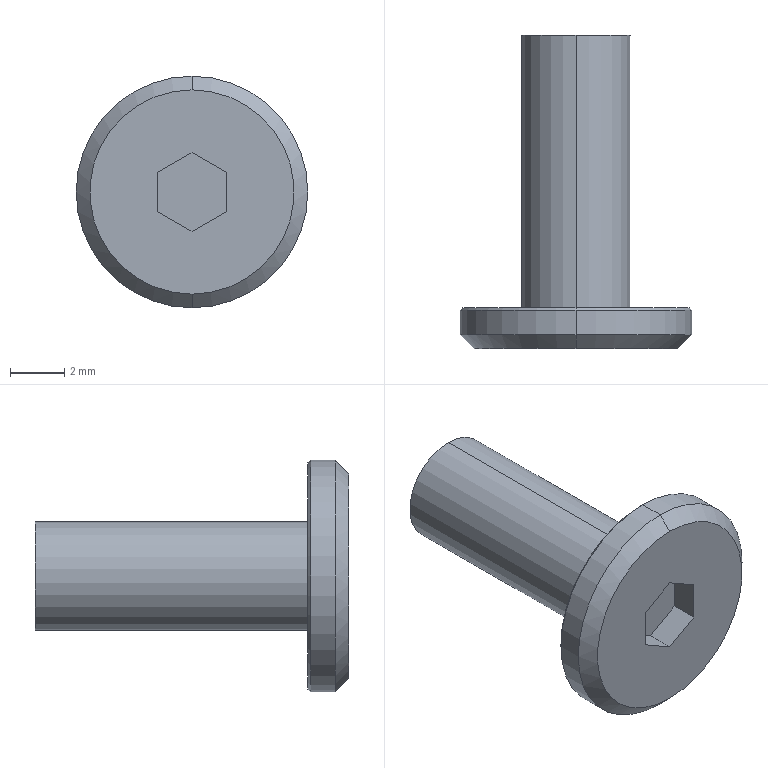Part | SolidWorks | features Chamfer 2, ICE 2, Extrusion 1, HoleWzd 1 | 1 solid | 22 faces | box 8.5 x 11.5 x 8.5 mm | volume 159.076 mm3 | plane 10 | cone 6 | cylinder 6 | commonest cylinder face diameters 2.5 x2 4 x2 8.5 x2
STEP:
#1=CARTESIAN_POINT('',(0.,1.5,4.15));
#2=VERTEX_POINT('',#1);
#3=CARTESIAN_POINT('',(0.,1.5,-4.15));
#4=VERTEX_POINT('',#3);
#5=CARTESIAN_POINT('',(0.,1.5,0.));
#6=DIRECTION('',(0.,1.,0.));
#7=DIRECTION('',(0.,0.,1.));
#8=AXIS2_PLACEMENT_3D('',#5,#6,#7);
#9=CIRCLE('',#8,4.15);
#10=EDGE_CURVE('',#2,#4,#9,.T.);
#11=ORIENTED_EDGE('',*,*,#10,.F.);
#12=CARTESIAN_POINT('',(0.,1.4,4.25));
#13=VERTEX_POINT('',#12);
#14=CARTESIAN_POINT('',(0.,1.5,4.15));
#15=DIRECTION('',(0.,-0.7071,0.7071));
#16=VECTOR('',#15,1000.);
#17=LINE('',#14,#16);
#18=EDGE_CURVE('',#2,#13,#17,.T.);
#19=ORIENTED_EDGE('',*,*,#18,.T.);
#20=CARTESIAN_POINT('',(0.,1.4,-4.25));
#21=VERTEX_POINT('',#20);
#22=CARTESIAN_POINT('',(0.,1.4,0.));
#23=DIRECTION('',(0.,-1.,0.));
#24=DIRECTION('',(0.,0.,1.));
#25=AXIS2_PLACEMENT_3D('',#22,#23,#24);
#26=CIRCLE('',#25,4.25);
#27=EDGE_CURVE('',#21,#13,#26,.T.);
#28=ORIENTED_EDGE('',*,*,#27,.F.);
#29=CARTESIAN_POINT('',(0.,1.5,-4.15));
#30=DIRECTION('',(0.,-0.7071,-0.7071));
#31=VECTOR('',#30,1000.);
#32=LINE('',#29,#31);
#33=EDGE_CURVE('',#4,#21,#32,.T.);
#34=ORIENTED_EDGE('',*,*,#33,.F.);
#35=EDGE_LOOP('',(#11,#19,#28,#34));
#36=FACE_OUTER_BOUND('',#35,.T.);
#37=CARTESIAN_POINT('',(0.,1.5,0.));
#38=DIRECTION('',(0.,-1.,0.));
#39=DIRECTION('',(0.,0.,-1.));
#40=AXIS2_PLACEMENT_3D('',#37,#38,#39);
#41=CONICAL_SURFACE('',#40,4.15,0.7854);
#42=ADVANCED_FACE('',(#36),#41,.T.);
#43=CARTESIAN_POINT('',(0.,0.,-3.75));
#44=VERTEX_POINT('',#43);
#45=CARTESIAN_POINT('',(0.,0.,3.75));
#46=VERTEX_POINT('',#45);
#47=CARTESIAN_POINT('',(0.,0.,0.));
#48=DIRECTION('',(0.,-1.,0.));
#49=DIRECTION('',(0.,0.,1.));
#50=AXIS2_PLACEMENT_3D('',#47,#48,#49);
#51=CIRCLE('',#50,3.75);
#52=EDGE_CURVE('',#44,#46,#51,.T.);
#53=ORIENTED_EDGE('',*,*,#52,.F.);
#54=CARTESIAN_POINT('',(0.,0.5,-4.25));
#55=VERTEX_POINT('',#54);
#56=CARTESIAN_POINT('',(0.,0.5,-4.25));
#57=DIRECTION('',(0.,0.7071,-0.7071));
#58=VECTOR('',#57,1000.);
#59=LINE('',#56,#58);
#60=EDGE_CURVE('',#44,#55,#59,.T.);
#61=ORIENTED_EDGE('',*,*,#60,.T.);
#62=CARTESIAN_POINT('',(0.,0.5,4.25));
#63=VERTEX_POINT('',#62);
#64=CARTESIAN_POINT('',(0.,0.5,0.));
#65=DIRECTION('',(0.,1.,0.));
#66=DIRECTION('',(0.,0.,1.));
#67=AXIS2_PLACEMENT_3D('',#64,#65,#66);
#68=CIRCLE('',#67,4.25);
#69=EDGE_CURVE('',#63,#55,#68,.T.);
#70=ORIENTED_EDGE('',*,*,#69,.F.);
#71=CARTESIAN_POINT('',(0.,0.5,4.25));
#72=DIRECTION('',(0.,0.7071,0.7071));
#73=VECTOR('',#72,1000.);
#74=LINE('',#71,#73);
#75=EDGE_CURVE('',#46,#63,#74,.T.);
#76=ORIENTED_EDGE('',*,*,#75,.F.);
#77=EDGE_LOOP('',(#53,#61,#70,#76));
#78=FACE_OUTER_BOUND('',#77,.T.);
#79=CARTESIAN_POINT('',(0.,0.5,0.));
#80=DIRECTION('',(0.,1.,0.));
#81=DIRECTION('',(0.,0.,1.));
#82=AXIS2_PLACEMENT_3D('',#79,#80,#81);
#83=CONICAL_SURFACE('',#82,4.25,0.7854);
#84=ADVANCED_FACE('',(#78),#83,.T.);
#85=CARTESIAN_POINT('',(0.,3.,-1.25));
#86=VERTEX_POINT('',#85);
#87=CARTESIAN_POINT('',(0.,3.,1.25));
#88=VERTEX_POINT('',#87);
#89=CARTESIAN_POINT('',(0.,3.,0.));
#90=DIRECTION('',(0.,1.,0.));
#91=DIRECTION('',(0.,0.,1.));
#92=AXIS2_PLACEMENT_3D('',#89,#90,#91);
#93=CIRCLE('',#92,1.25);
#94=EDGE_CURVE('',#86,#88,#93,.T.);
#95=ORIENTED_EDGE('',*,*,#94,.F.);
#96=CARTESIAN_POINT('',(0.,11.5,-1.25));
#97=VERTEX_POINT('',#96);
#98=CARTESIAN_POINT('',(0.,11.5,-1.25));
#99=DIRECTION('',(0.,1.,0.));
#100=VECTOR('',#99,1000.);
#101=LINE('',#98,#100);
#102=EDGE_CURVE('',#86,#97,#101,.T.);
#103=ORIENTED_EDGE('',*,*,#102,.T.);
#104=CARTESIAN_POINT('',(0.,11.5,1.25));
#105=VERTEX_POINT('',#104);
#106=CARTESIAN_POINT('',(0.,11.5,0.));
#107=DIRECTION('',(0.,1.,0.));
#108=DIRECTION('',(0.,0.,1.));
#109=AXIS2_PLACEMENT_3D('',#106,#107,#108);
#110=CIRCLE('',#109,1.25);
#111=EDGE_CURVE('',#97,#105,#110,.T.);
#112=ORIENTED_EDGE('',*,*,#111,.T.);
#113=CARTESIAN_POINT('',(0.,11.5,1.25));
#114=DIRECTION('',(0.,1.,0.));
#115=VECTOR('',#114,1000.);
#116=LINE('',#113,#115);
#117=EDGE_CURVE('',#88,#105,#116,.T.);
#118=ORIENTED_EDGE('',*,*,#117,.F.);
#119=EDGE_LOOP('',(#95,#103,#112,#118));
#120=FACE_OUTER_BOUND('',#119,.T.);
#121=CARTESIAN_POINT('',(0.,11.5,0.));
#122=DIRECTION('',(0.,1.,0.));
#123=DIRECTION('',(0.,0.,1.));
#124=AXIS2_PLACEMENT_3D('',#121,#122,#123);
#125=CYLINDRICAL_SURFACE('',#124,1.25);
#126=ADVANCED_FACE('',(#120),#125,.F.);
#127=CARTESIAN_POINT('',(0.,2.249,0.));
#128=VERTEX_POINT('',#127);
#129=CARTESIAN_POINT('',(0.,3.,1.25));
#130=DIRECTION('',(0.,0.515,0.8572));
#131=VECTOR('',#130,1000.);
#132=LINE('',#129,#131);
#133=EDGE_CURVE('',#128,#88,#132,.T.);
#134=ORIENTED_EDGE('',*,*,#133,.F.);
#135=CARTESIAN_POINT('',(0.,3.,-1.25));
#136=DIRECTION('',(0.,0.515,-0.8572));
#137=VECTOR('',#136,1000.);
#138=LINE('',#135,#137);
#139=EDGE_CURVE('',#128,#86,#138,.T.);
#140=ORIENTED_EDGE('',*,*,#139,.T.);
#141=ORIENTED_EDGE('',*,*,#94,.T.);
#142=EDGE_LOOP('',(#134,#140,#141));
#143=FACE_OUTER_BOUND('',#142,.T.);
#144=CARTESIAN_POINT('',(0.,3.,0.));
#145=DIRECTION('',(0.,1.,0.));
#146=DIRECTION('',(0.,0.,1.));
#147=AXIS2_PLACEMENT_3D('',#144,#145,#146);
#148=CONICAL_SURFACE('',#147,1.25,1.03);
#149=ADVANCED_FACE('',(#143),#148,.F.);
#150=CARTESIAN_POINT('',(0.,11.5,2.));
#151=VERTEX_POINT('',#150);
#152=CARTESIAN_POINT('',(0.,11.5,-2.));
#153=VERTEX_POINT('',#152);
#154=CARTESIAN_POINT('',(0.,11.5,0.));
#155=DIRECTION('',(0.,1.,0.));
#156=DIRECTION('',(0.,0.,1.));
#157=AXIS2_PLACEMENT_3D('',#154,#155,#156);
#158=CIRCLE('',#157,2.);
#159=EDGE_CURVE('',#151,#153,#158,.T.);
#160=ORIENTED_EDGE('',*,*,#159,.F.);
#161=CARTESIAN_POINT('',(0.,1.5,2.));
#162=VERTEX_POINT('',#161);
#163=CARTESIAN_POINT('',(0.,11.5,2.));
#164=DIRECTION('',(0.,-1.,0.));
#165=VECTOR('',#164,1000.);
#166=LINE('',#163,#165);
#167=EDGE_CURVE('',#151,#162,#166,.T.);
#168=ORIENTED_EDGE('',*,*,#167,.T.);
#169=CARTESIAN_POINT('',(0.,1.5,-2.));
#170=VERTEX_POINT('',#169);
#171=CARTESIAN_POINT('',(0.,1.5,0.));
#172=DIRECTION('',(0.,1.,0.));
#173=DIRECTION('',(0.,0.,1.));
#174=AXIS2_PLACEMENT_3D('',#171,#172,#173);
#175=CIRCLE('',#174,2.);
#176=EDGE_CURVE('',#162,#170,#175,.T.);
#177=ORIENTED_EDGE('',*,*,#176,.T.);
#178=CARTESIAN_POINT('',(0.,11.5,-2.));
#179=DIRECTION('',(0.,-1.,0.));
#180=VECTOR('',#179,1000.);
#181=LINE('',#178,#180);
#182=EDGE_CURVE('',#153,#170,#181,.T.);
#183=ORIENTED_EDGE('',*,*,#182,.F.);
#184=EDGE_LOOP('',(#160,#168,#177,#183));
#185=FACE_OUTER_BOUND('',#184,.T.);
#186=CARTESIAN_POINT('',(0.,11.5,0.));
#187=DIRECTION('',(0.,-1.,0.));
#188=DIRECTION('',(0.,0.,-1.));
#189=AXIS2_PLACEMENT_3D('',#186,#187,#188);
#190=CYLINDRICAL_SURFACE('',#189,2.);
#191=ADVANCED_FACE('',(#185),#190,.T.);
#192=ORIENTED_EDGE('',*,*,#27,.T.);
#193=CARTESIAN_POINT('',(0.,1.5,4.25));
#194=DIRECTION('',(0.,-1.,0.));
#195=VECTOR('',#194,1000.);
#196=LINE('',#193,#195);
#197=EDGE_CURVE('',#13,#63,#196,.T.);
#198=ORIENTED_EDGE('',*,*,#197,.T.);
#199=ORIENTED_EDGE('',*,*,#69,.T.);
#200=CARTESIAN_POINT('',(0.,1.5,-4.25));
#201=DIRECTION('',(0.,-1.,0.));
#202=VECTOR('',#201,1000.);
#203=LINE('',#200,#202);
#204=EDGE_CURVE('',#21,#55,#203,.T.);
#205=ORIENTED_EDGE('',*,*,#204,.F.);
#206=EDGE_LOOP('',(#192,#198,#199,#205));
#207=FACE_OUTER_BOUND('',#206,.T.);
#208=CARTESIAN_POINT('',(0.,1.5,0.));
#209=DIRECTION('',(0.,-1.,0.));
#210=DIRECTION('',(0.,0.,-1.));
#211=AXIS2_PLACEMENT_3D('',#208,#209,#210);
#212=CYLINDRICAL_SURFACE('',#211,4.25);
#213=ADVANCED_FACE('',(#207),#212,.T.);
#214=ORIENTED_EDGE('',*,*,#197,.F.);
#215=CARTESIAN_POINT('',(0.,1.4,0.));
#216=DIRECTION('',(0.,-1.,0.));
#217=DIRECTION('',(0.,0.,1.));
#218=AXIS2_PLACEMENT_3D('',#215,#216,#217);
#219=CIRCLE('',#218,4.25);
#220=EDGE_CURVE('',#13,#21,#219,.T.);
#221=ORIENTED_EDGE('',*,*,#220,.T.);
#222=ORIENTED_EDGE('',*,*,#204,.T.);
#223=CARTESIAN_POINT('',(0.,0.5,0.));
#224=DIRECTION('',(0.,1.,0.));
#225=DIRECTION('',(0.,0.,1.));
#226=AXIS2_PLACEMENT_3D('',#223,#224,#225);
#227=CIRCLE('',#226,4.25);
#228=EDGE_CURVE('',#55,#63,#227,.T.);
#229=ORIENTED_EDGE('',*,*,#228,.T.);
#230=EDGE_LOOP('',(#214,#221,#222,#229));
#231=FACE_OUTER_BOUND('',#230,.T.);
#232=CARTESIAN_POINT('',(0.,1.5,0.));
#233=DIRECTION('',(0.,-1.,0.));
#234=DIRECTION('',(0.,0.,-1.));
#235=AXIS2_PLACEMENT_3D('',#232,#233,#234);
#236=CYLINDRICAL_SURFACE('',#235,4.25);
#237=ADVANCED_FACE('',(#231),#236,.T.);
#238=CARTESIAN_POINT('',(0.,1.5,0.));
#239=DIRECTION('',(0.,1.,0.));
#240=DIRECTION('',(0.,0.,1.));
#241=AXIS2_PLACEMENT_3D('',#238,#239,#240);
#242=CIRCLE('',#241,4.15);
#243=EDGE_CURVE('',#4,#2,#242,.T.);
#244=ORIENTED_EDGE('',*,*,#243,.T.);
#245=ORIENTED_EDGE('',*,*,#10,.T.);
#246=EDGE_LOOP('',(#244,#245));
#247=FACE_OUTER_BOUND('',#246,.T.);
#248=CARTESIAN_POINT('',(0.,1.5,0.));
#249=DIRECTION('',(0.,1.,0.));
#250=DIRECTION('',(0.,0.,1.));
#251=AXIS2_PLACEMENT_3D('',#248,#249,#250);
#252=CIRCLE('',#251,2.);
#253=EDGE_CURVE('',#170,#162,#252,.T.);
#254=ORIENTED_EDGE('',*,*,#253,.F.);
#255=ORIENTED_EDGE('',*,*,#176,.F.);
#256=EDGE_LOOP('',(#254,#255));
#257=FACE_BOUND('',#256,.T.);
#258=CARTESIAN_POINT('',(0.,1.5,0.));
#259=DIRECTION('',(0.,1.,0.));
#260=DIRECTION('',(0.,0.,1.));
#261=AXIS2_PLACEMENT_3D('',#258,#259,#260);
#262=PLANE('',#261);
#263=ADVANCED_FACE('',(#247,#257),#262,.T.);
#264=CARTESIAN_POINT('',(0.,0.,0.));
#265=DIRECTION('',(0.,-1.,0.));
#266=DIRECTION('',(0.,0.,1.));
#267=AXIS2_PLACEMENT_3D('',#264,#265,#266);
#268=CIRCLE('',#267,3.75);
#269=EDGE_CURVE('',#46,#44,#268,.T.);
#270=ORIENTED_EDGE('',*,*,#269,.T.);
#271=ORIENTED_EDGE('',*,*,#52,.T.);
#272=EDGE_LOOP('',(#270,#271));
#273=FACE_OUTER_BOUND('',#272,.T.);
#274=CARTESIAN_POINT('',(0.,0.,1.443));
#275=VERTEX_POINT('',#274);
#276=CARTESIAN_POINT('',(-1.25,0.,0.7217));
#277=VERTEX_POINT('',#276);
#278=CARTESIAN_POINT('',(0.,0.,1.443));
#279=DIRECTION('',(-0.866,0.,-0.5));
#280=VECTOR('',#279,1000.);
#281=LINE('',#278,#280);
#282=EDGE_CURVE('',#275,#277,#281,.T.);
#283=ORIENTED_EDGE('',*,*,#282,.F.);
#284=CARTESIAN_POINT('',(1.25,0.,0.7217));
#285=VERTEX_POINT('',#284);
#286=CARTESIAN_POINT('',(1.25,0.,0.7217));
#287=DIRECTION('',(-0.866,0.,0.5));
#288=VECTOR('',#287,1000.);
#289=LINE('',#286,#288);
#290=EDGE_CURVE('',#285,#275,#289,.T.);
#291=ORIENTED_EDGE('',*,*,#290,.F.);
#292=CARTESIAN_POINT('',(1.25,0.,-0.7217));
#293=VERTEX_POINT('',#292);
#294=CARTESIAN_POINT('',(1.25,0.,-0.7217));
#295=DIRECTION('',(0.,0.,1.));
#296=VECTOR('',#295,1000.);
#297=LINE('',#294,#296);
#298=EDGE_CURVE('',#293,#285,#297,.T.);
#299=ORIENTED_EDGE('',*,*,#298,.F.);
#300=CARTESIAN_POINT('',(0.,0.,-1.443));
#301=VERTEX_POINT('',#300);
#302=CARTESIAN_POINT('',(0.,0.,-1.443));
#303=DIRECTION('',(0.866,0.,0.5));
#304=VECTOR('',#303,1000.);
#305=LINE('',#302,#304);
#306=EDGE_CURVE('',#301,#293,#305,.T.);
#307=ORIENTED_EDGE('',*,*,#306,.F.);
#308=CARTESIAN_POINT('',(-1.25,0.,-0.7217));
#309=VERTEX_POINT('',#308);
#310=CARTESIAN_POINT('',(-1.25,0.,-0.7217));
#311=DIRECTION('',(0.866,0.,-0.5));
#312=VECTOR('',#311,1000.);
#313=LINE('',#310,#312);
#314=EDGE_CURVE('',#309,#301,#313,.T.);
#315=ORIENTED_EDGE('',*,*,#314,.F.);
#316=CARTESIAN_POINT('',(-1.25,0.,0.7217));
#317=DIRECTION('',(0.,0.,-1.));
#318=VECTOR('',#317,1000.);
#319=LINE('',#316,#318);
#320=EDGE_CURVE('',#277,#309,#319,.T.);
#321=ORIENTED_EDGE('',*,*,#320,.F.);
#322=EDGE_LOOP('',(#283,#291,#299,#307,#315,#321));
#323=FACE_BOUND('',#322,.T.);
#324=CARTESIAN_POINT('',(0.,0.,0.));
#325=DIRECTION('',(0.,1.,0.));
#326=DIRECTION('',(0.,0.,1.));
#327=AXIS2_PLACEMENT_3D('',#324,#325,#326);
#328=PLANE('',#327);
#329=ADVANCED_FACE('',(#273,#323),#328,.F.);
#330=ORIENTED_EDGE('',*,*,#167,.F.);
#331=CARTESIAN_POINT('',(0.,11.5,0.));
#332=DIRECTION('',(0.,1.,0.));
#333=DIRECTION('',(0.,0.,1.));
#334=AXIS2_PLACEMENT_3D('',#331,#332,#333);
#335=CIRCLE('',#334,2.);
#336=EDGE_CURVE('',#153,#151,#335,.T.);
#337=ORIENTED_EDGE('',*,*,#336,.F.);
#338=ORIENTED_EDGE('',*,*,#182,.T.);
#339=ORIENTED_EDGE('',*,*,#253,.T.);
#340=EDGE_LOOP('',(#330,#337,#338,#339));
#341=FACE_OUTER_BOUND('',#340,.T.);
#342=CARTESIAN_POINT('',(0.,11.5,0.));
#343=DIRECTION('',(0.,-1.,0.));
#344=DIRECTION('',(0.,0.,-1.));
#345=AXIS2_PLACEMENT_3D('',#342,#343,#344);
#346=CYLINDRICAL_SURFACE('',#345,2.);
#347=ADVANCED_FACE('',(#341),#346,.T.);
#348=CARTESIAN_POINT('',(0.,11.5,0.));
#349=DIRECTION('',(0.,1.,0.));
#350=DIRECTION('',(0.,0.,1.));
#351=AXIS2_PLACEMENT_3D('',#348,#349,#350);
#352=CIRCLE('',#351,1.25);
#353=EDGE_CURVE('',#105,#97,#352,.T.);
#354=ORIENTED_EDGE('',*,*,#353,.F.);
#355=ORIENTED_EDGE('',*,*,#111,.F.);
#356=EDGE_LOOP('',(#354,#355));
#357=FACE_BOUND('',#356,.T.);
#358=ORIENTED_EDGE('',*,*,#336,.T.);
#359=ORIENTED_EDGE('',*,*,#159,.T.);
#360=EDGE_LOOP('',(#358,#359));
#361=FACE_OUTER_BOUND('',#360,.T.);
#362=CARTESIAN_POINT('',(0.,11.5,0.));
#363=DIRECTION('',(0.,1.,0.));
#364=DIRECTION('',(0.,0.,1.));
#365=AXIS2_PLACEMENT_3D('',#362,#363,#364);
#366=PLANE('',#365);
#367=ADVANCED_FACE('',(#357,#361),#366,.T.);
#368=ORIENTED_EDGE('',*,*,#139,.F.);
#369=ORIENTED_EDGE('',*,*,#133,.T.);
#370=CARTESIAN_POINT('',(0.,3.,0.));
#371=DIRECTION('',(0.,1.,0.));
#372=DIRECTION('',(0.,0.,1.));
#373=AXIS2_PLACEMENT_3D('',#370,#371,#372);
#374=CIRCLE('',#373,1.25);
#375=EDGE_CURVE('',#88,#86,#374,.T.);
#376=ORIENTED_EDGE('',*,*,#375,.T.);
#377=EDGE_LOOP('',(#368,#369,#376));
#378=FACE_OUTER_BOUND('',#377,.T.);
#379=CARTESIAN_POINT('',(0.,3.,0.));
#380=DIRECTION('',(0.,1.,0.));
#381=DIRECTION('',(0.,0.,1.));
#382=AXIS2_PLACEMENT_3D('',#379,#380,#381);
#383=CONICAL_SURFACE('',#382,1.25,1.03);
#384=ADVANCED_FACE('',(#378),#383,.F.);
#385=ORIENTED_EDGE('',*,*,#102,.F.);
#386=ORIENTED_EDGE('',*,*,#375,.F.);
#387=ORIENTED_EDGE('',*,*,#117,.T.);
#388=ORIENTED_EDGE('',*,*,#353,.T.);
#389=EDGE_LOOP('',(#385,#386,#387,#388));
#390=FACE_OUTER_BOUND('',#389,.T.);
#391=CARTESIAN_POINT('',(0.,11.5,0.));
#392=DIRECTION('',(0.,1.,0.));
#393=DIRECTION('',(0.,0.,1.));
#394=AXIS2_PLACEMENT_3D('',#391,#392,#393);
#395=CYLINDRICAL_SURFACE('',#394,1.25);
#396=ADVANCED_FACE('',(#390),#395,.F.);
#397=ORIENTED_EDGE('',*,*,#290,.T.);
#398=CARTESIAN_POINT('',(0.,1.,1.443));
#399=VERTEX_POINT('',#398);
#400=CARTESIAN_POINT('',(0.,1.,1.443));
#401=DIRECTION('',(0.,-1.,0.));
#402=VECTOR('',#401,1000.);
#403=LINE('',#400,#402);
#404=EDGE_CURVE('',#399,#275,#403,.T.);
#405=ORIENTED_EDGE('',*,*,#404,.F.);
#406=CARTESIAN_POINT('',(1.25,1.,0.7217));
#407=VERTEX_POINT('',#406);
#408=CARTESIAN_POINT('',(1.25,1.,0.7217));
#409=DIRECTION('',(-0.866,0.,0.5));
#410=VECTOR('',#409,1000.);
#411=LINE('',#408,#410);
#412=EDGE_CURVE('',#407,#399,#411,.T.);
#413=ORIENTED_EDGE('',*,*,#412,.F.);
#414=CARTESIAN_POINT('',(1.25,1.,0.7217));
#415=DIRECTION('',(0.,-1.,0.));
#416=VECTOR('',#415,1000.);
#417=LINE('',#414,#416);
#418=EDGE_CURVE('',#407,#285,#417,.T.);
#419=ORIENTED_EDGE('',*,*,#418,.T.);
#420=EDGE_LOOP('',(#397,#405,#413,#419));
#421=FACE_OUTER_BOUND('',#420,.T.);
#422=CARTESIAN_POINT('',(1.25,1.,0.7217));
#423=DIRECTION('',(0.5,0.,0.866));
#424=DIRECTION('',(0.866,0.,-0.5));
#425=AXIS2_PLACEMENT_3D('',#422,#423,#424);
#426=PLANE('',#425);
#427=ADVANCED_FACE('',(#421),#426,.F.);
#428=ORIENTED_EDGE('',*,*,#298,.T.);
#429=ORIENTED_EDGE('',*,*,#418,.F.);
#430=CARTESIAN_POINT('',(1.25,1.,-0.7217));
#431=VERTEX_POINT('',#430);
#432=CARTESIAN_POINT('',(1.25,1.,-0.7217));
#433=DIRECTION('',(0.,0.,1.));
#434=VECTOR('',#433,1000.);
#435=LINE('',#432,#434);
#436=EDGE_CURVE('',#431,#407,#435,.T.);
#437=ORIENTED_EDGE('',*,*,#436,.F.);
#438=CARTESIAN_POINT('',(1.25,1.,-0.7217));
#439=DIRECTION('',(0.,-1.,0.));
#440=VECTOR('',#439,1000.);
#441=LINE('',#438,#440);
#442=EDGE_CURVE('',#431,#293,#441,.T.);
#443=ORIENTED_EDGE('',*,*,#442,.T.);
#444=EDGE_LOOP('',(#428,#429,#437,#443));
#445=FACE_OUTER_BOUND('',#444,.T.);
#446=CARTESIAN_POINT('',(1.25,1.,-0.7217));
#447=DIRECTION('',(1.,0.,0.));
#448=DIRECTION('',(0.,0.,-1.));
#449=AXIS2_PLACEMENT_3D('',#446,#447,#448);
#450=PLANE('',#449);
#451=ADVANCED_FACE('',(#445),#450,.F.);
#452=ORIENTED_EDGE('',*,*,#306,.T.);
#453=ORIENTED_EDGE('',*,*,#442,.F.);
#454=CARTESIAN_POINT('',(0.,1.,-1.443));
#455=VERTEX_POINT('',#454);
#456=CARTESIAN_POINT('',(0.,1.,-1.443));
#457=DIRECTION('',(0.866,0.,0.5));
#458=VECTOR('',#457,1000.);
#459=LINE('',#456,#458);
#460=EDGE_CURVE('',#455,#431,#459,.T.);
#461=ORIENTED_EDGE('',*,*,#460,.F.);
#462=CARTESIAN_POINT('',(0.,1.,-1.443));
#463=DIRECTION('',(0.,-1.,0.));
#464=VECTOR('',#463,1000.);
#465=LINE('',#462,#464);
#466=EDGE_CURVE('',#455,#301,#465,.T.);
#467=ORIENTED_EDGE('',*,*,#466,.T.);
#468=EDGE_LOOP('',(#452,#453,#461,#467));
#469=FACE_OUTER_BOUND('',#468,.T.);
#470=CARTESIAN_POINT('',(0.,1.,-1.443));
#471=DIRECTION('',(0.5,0.,-0.866));
#472=DIRECTION('',(-0.866,0.,-0.5));
#473=AXIS2_PLACEMENT_3D('',#470,#471,#472);
#474=PLANE('',#473);
#475=ADVANCED_FACE('',(#469),#474,.F.);
#476=ORIENTED_EDGE('',*,*,#314,.T.);
#477=ORIENTED_EDGE('',*,*,#466,.F.);
#478=CARTESIAN_POINT('',(-1.25,1.,-0.7217));
#479=VERTEX_POINT('',#478);
#480=CARTESIAN_POINT('',(-1.25,1.,-0.7217));
#481=DIRECTION('',(0.866,0.,-0.5));
#482=VECTOR('',#481,1000.);
#483=LINE('',#480,#482);
#484=EDGE_CURVE('',#479,#455,#483,.T.);
#485=ORIENTED_EDGE('',*,*,#484,.F.);
#486=CARTESIAN_POINT('',(-1.25,1.,-0.7217));
#487=DIRECTION('',(0.,-1.,0.));
#488=VECTOR('',#487,1000.);
#489=LINE('',#486,#488);
#490=EDGE_CURVE('',#479,#309,#489,.T.);
#491=ORIENTED_EDGE('',*,*,#490,.T.);
#492=EDGE_LOOP('',(#476,#477,#485,#491));
#493=FACE_OUTER_BOUND('',#492,.T.);
#494=CARTESIAN_POINT('',(-1.25,1.,-0.7217));
#495=DIRECTION('',(-0.5,0.,-0.866));
#496=DIRECTION('',(-0.866,0.,0.5));
#497=AXIS2_PLACEMENT_3D('',#494,#495,#496);
#498=PLANE('',#497);
#499=ADVANCED_FACE('',(#493),#498,.F.);
#500=ORIENTED_EDGE('',*,*,#320,.T.);
#501=ORIENTED_EDGE('',*,*,#490,.F.);
#502=CARTESIAN_POINT('',(-1.25,1.,0.7217));
#503=VERTEX_POINT('',#502);
#504=CARTESIAN_POINT('',(-1.25,1.,0.7217));
#505=DIRECTION('',(0.,0.,-1.));
#506=VECTOR('',#505,1000.);
#507=LINE('',#504,#506);
#508=EDGE_CURVE('',#503,#479,#507,.T.);
#509=ORIENTED_EDGE('',*,*,#508,.F.);
#510=CARTESIAN_POINT('',(-1.25,1.,0.7217));
#511=DIRECTION('',(0.,-1.,0.));
#512=VECTOR('',#511,1000.);
#513=LINE('',#510,#512);
#514=EDGE_CURVE('',#503,#277,#513,.T.);
#515=ORIENTED_EDGE('',*,*,#514,.T.);
#516=EDGE_LOOP('',(#500,#501,#509,#515));
#517=FACE_OUTER_BOUND('',#516,.T.);
#518=CARTESIAN_POINT('',(-1.25,1.,0.7217));
#519=DIRECTION('',(-1.,0.,0.));
#520=DIRECTION('',(0.,0.,1.));
#521=AXIS2_PLACEMENT_3D('',#518,#519,#520);
#522=PLANE('',#521);
#523=ADVANCED_FACE('',(#517),#522,.F.);
#524=ORIENTED_EDGE('',*,*,#282,.T.);
#525=ORIENTED_EDGE('',*,*,#514,.F.);
#526=CARTESIAN_POINT('',(0.,1.,1.443));
#527=DIRECTION('',(-0.866,0.,-0.5));
#528=VECTOR('',#527,1000.);
#529=LINE('',#526,#528);
#530=EDGE_CURVE('',#399,#503,#529,.T.);
#531=ORIENTED_EDGE('',*,*,#530,.F.);
#532=ORIENTED_EDGE('',*,*,#404,.T.);
#533=EDGE_LOOP('',(#524,#525,#531,#532));
#534=FACE_OUTER_BOUND('',#533,.T.);
#535=CARTESIAN_POINT('',(0.,1.,1.443));
#536=DIRECTION('',(-0.5,0.,0.866));
#537=DIRECTION('',(0.866,0.,0.5));
#538=AXIS2_PLACEMENT_3D('',#535,#536,#537);
#539=PLANE('',#538);
#540=ADVANCED_FACE('',(#534),#539,.F.);
#541=ORIENTED_EDGE('',*,*,#412,.T.);
#542=ORIENTED_EDGE('',*,*,#530,.T.);
#543=ORIENTED_EDGE('',*,*,#508,.T.);
#544=ORIENTED_EDGE('',*,*,#484,.T.);
#545=ORIENTED_EDGE('',*,*,#460,.T.);
#546=ORIENTED_EDGE('',*,*,#436,.T.);
#547=EDGE_LOOP('',(#541,#542,#543,#544,#545,#546));
#548=FACE_OUTER_BOUND('',#547,.T.);
#549=CARTESIAN_POINT('',(0.,1.,0.));
#550=DIRECTION('',(0.,-1.,0.));
#551=DIRECTION('',(0.,0.,-1.));
#552=AXIS2_PLACEMENT_3D('',#549,#550,#551);
#553=PLANE('',#552);
#554=ADVANCED_FACE('',(#548),#553,.T.);
#555=ORIENTED_EDGE('',*,*,#60,.F.);
#556=ORIENTED_EDGE('',*,*,#269,.F.);
#557=ORIENTED_EDGE('',*,*,#75,.T.);
#558=ORIENTED_EDGE('',*,*,#228,.F.);
#559=EDGE_LOOP('',(#555,#556,#557,#558));
#560=FACE_OUTER_BOUND('',#559,.T.);
#561=CARTESIAN_POINT('',(0.,0.5,0.));
#562=DIRECTION('',(0.,1.,0.));
#563=DIRECTION('',(0.,0.,1.));
#564=AXIS2_PLACEMENT_3D('',#561,#562,#563);
#565=CONICAL_SURFACE('',#564,4.25,0.7854);
#566=ADVANCED_FACE('',(#560),#565,.T.);
#567=ORIENTED_EDGE('',*,*,#18,.F.);
#568=ORIENTED_EDGE('',*,*,#243,.F.);
#569=ORIENTED_EDGE('',*,*,#33,.T.);
#570=ORIENTED_EDGE('',*,*,#220,.F.);
#571=EDGE_LOOP('',(#567,#568,#569,#570));
#572=FACE_OUTER_BOUND('',#571,.T.);
#573=CARTESIAN_POINT('',(0.,1.5,0.));
#574=DIRECTION('',(0.,-1.,0.));
#575=DIRECTION('',(0.,0.,-1.));
#576=AXIS2_PLACEMENT_3D('',#573,#574,#575);
#577=CONICAL_SURFACE('',#576,4.15,0.7854);
#578=ADVANCED_FACE('',(#572),#577,.T.);
#579=CLOSED_SHELL('',(#42,#84,#126,#149,#191,#213,#237,#263,#329,#347,#367,#384,#396,#427,#451,#475,#499,#523,#540,#554,#566,#578));
#580=MANIFOLD_SOLID_BREP('',#579);
#581=CARTESIAN_POINT('',(0.,0.,0.));
#582=DIRECTION('',(0.,0.,1.));
#583=DIRECTION('',(1.,0.,0.));
#584=AXIS2_PLACEMENT_3D('',#581,#582,#583);
#585=(LENGTH_UNIT()NAMED_UNIT(*)SI_UNIT(.MILLI.,.METRE.));
#586=UNCERTAINTY_MEASURE_WITH_UNIT(LENGTH_MEASURE(0.00001),#585,'','');
#587=(NAMED_UNIT(*)PLANE_ANGLE_UNIT()SI_UNIT($,.RADIAN.));
#588=(NAMED_UNIT(*)SI_UNIT($,.STERADIAN.)SOLID_ANGLE_UNIT());
#589=(GEOMETRIC_REPRESENTATION_CONTEXT(3)GLOBAL_UNCERTAINTY_ASSIGNED_CONTEXT((#586))GLOBAL_UNIT_ASSIGNED_CONTEXT((#585,#587,#588))REPRESENTATION_CONTEXT('',''));
#590=ADVANCED_BREP_SHAPE_REPRESENTATION('',(#580,#584),#589);